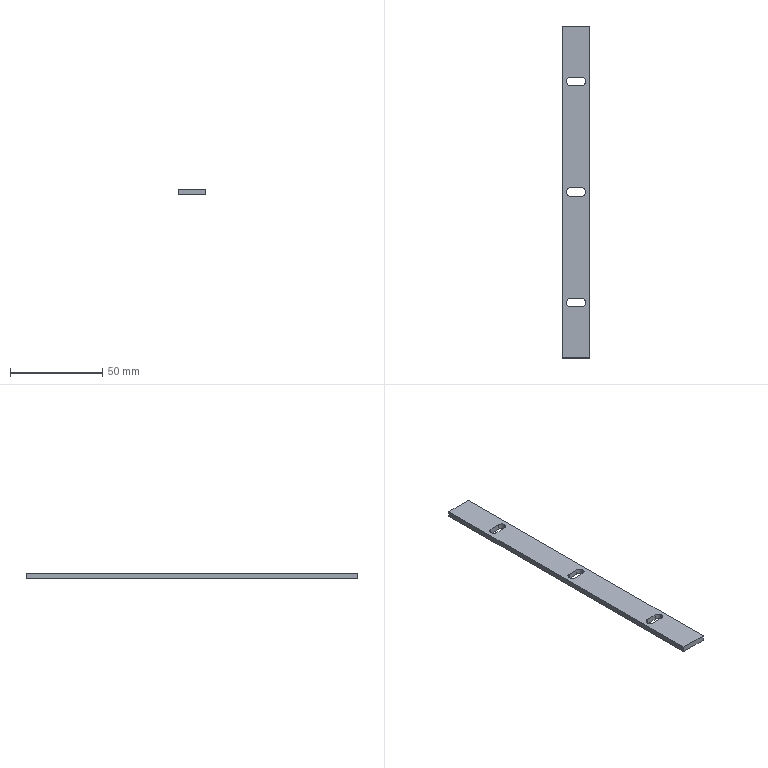Part | STEP file | PN_0041 Mount electronic clip pressure rod | 1 solid | 21 faces | box 15 x 180 x 3 mm | volume 7714 mm3 | plane 12 | cylinder 9 | commonest cylinder face diameters 4.5 x9